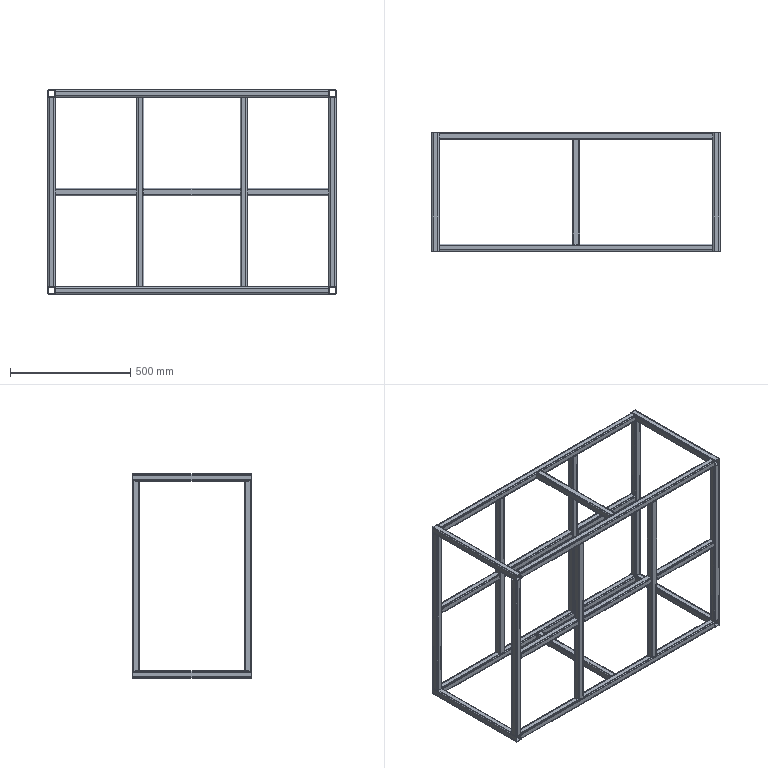Part | SolidWorks | features WeldCornerFeat 2, 3DProfileFeature 1, WeldMemberFeat 1, WeldmentFeature 1 | 24 solids | 432 faces | box 1200 x 495 x 850 mm | volume 4251393 mm3 | plane 240 | cylinder 192 | commonest cylinder face diameters 5.2 x96 10.4 x96